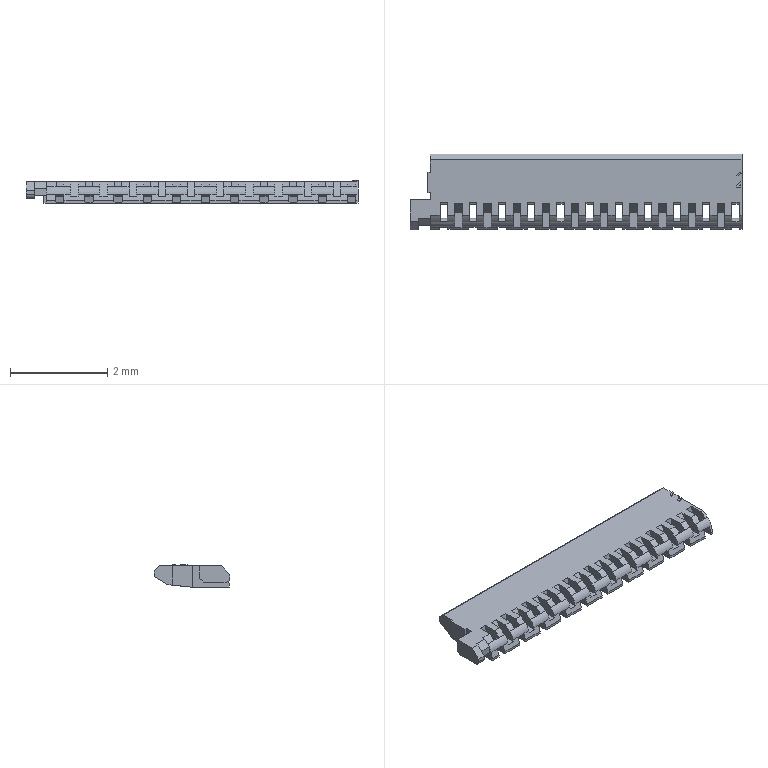Part | Creo | 1 solid | 238 faces | box 6.83 x 1.56 x 0.4631 mm | volume 3.381 mm3 | plane 193 | cylinder 45 | commonest cylinder face diameters 1.165 x22 0.2 x11 0.39 x11 0.16 x1